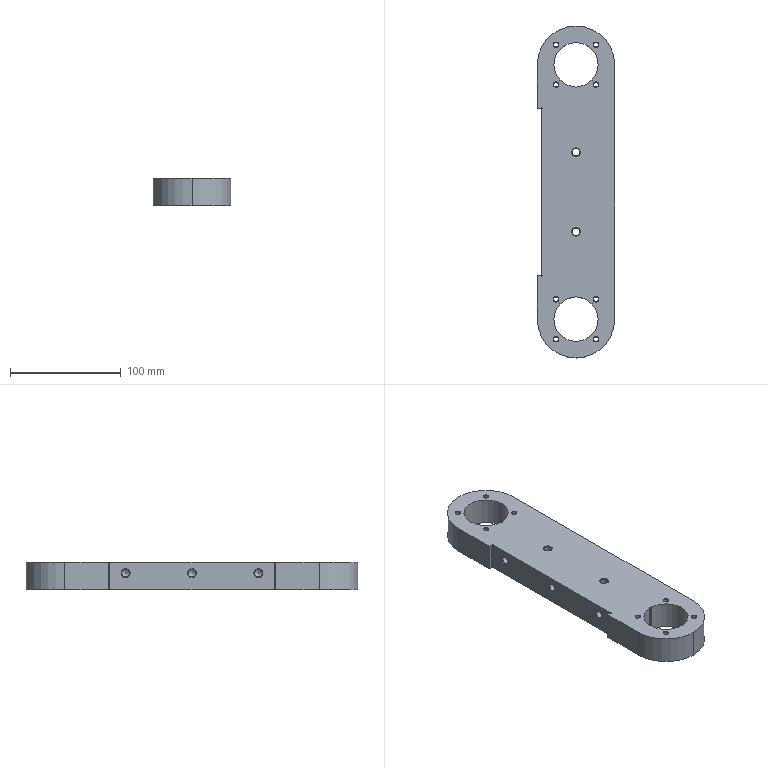Part | STEP file | YBQDJ-QD-6 | 1 solid | 65 faces | box 70 x 300 x 25 mm | volume 414235 mm3 | cylinder 31 | cone 26 | plane 8 | commonest cylinder face diameters 4.2 x8 6.8 x5 1 x4 2 x4 4 x4 70 x4